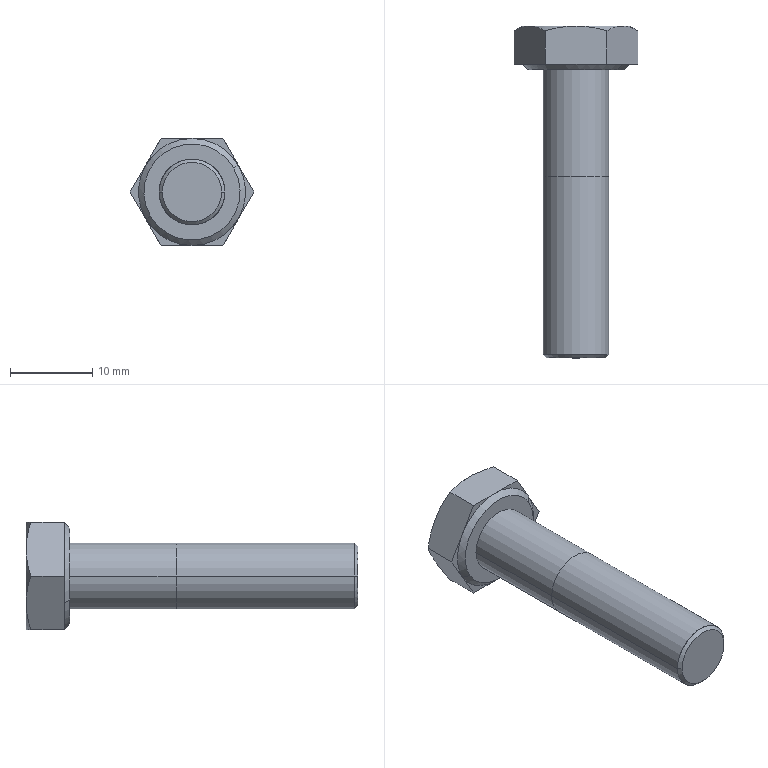Part | NX | features BREP 2 | 1 solid | 31 faces | box 15.011 x 40.3 x 13 mm | volume 2901 mm3 | plane 17 | cone 10 | cylinder 4 | commonest cylinder face diameters 6.647 x2 8 x2